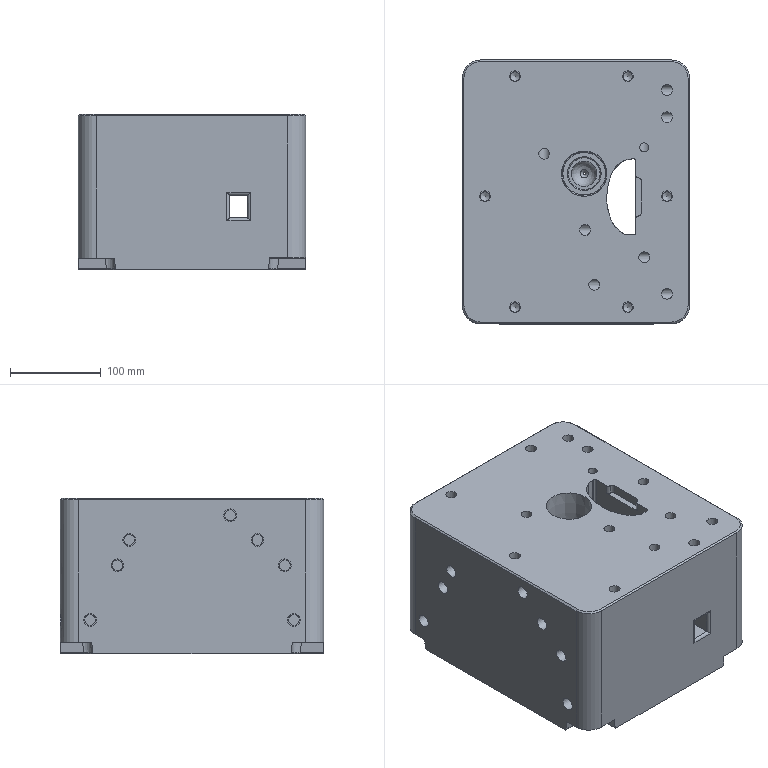Part | STEP file | solid 159 | 1 solid | 974 faces | box 250 x 290 x 170.5 mm | volume 8891009 mm3 | spline 335 | cylinder 257 | plane 216 | torus 78 | cone 46 | sphere 35 | other 7 | commonest cylinder face diameters 1.005 x56 12 x34 0.603 x20 6 x16 5.025 x15 8.04 x13